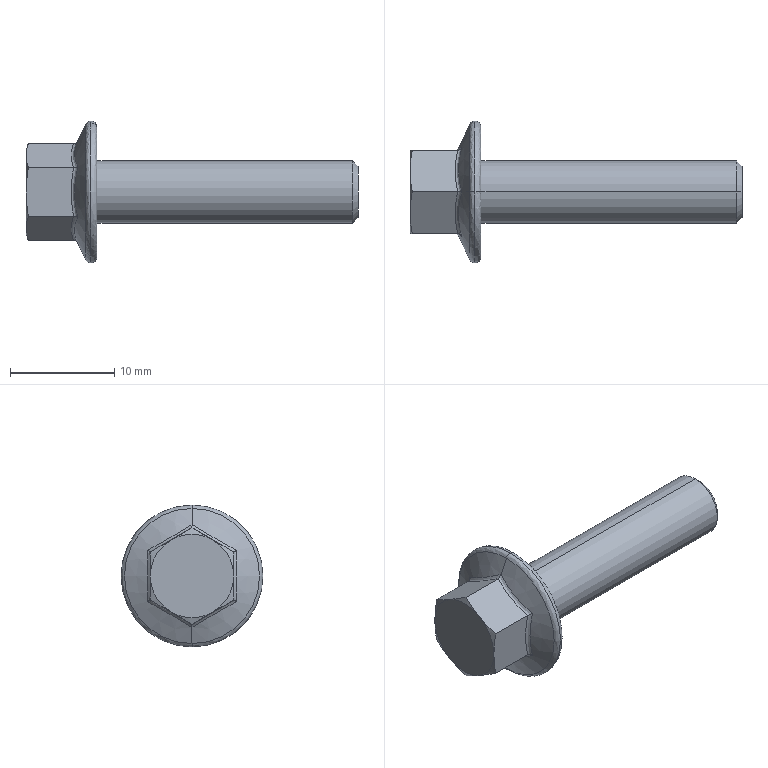Part | STEP file | hexagon flange bolts--small series gb_PreviewCfg | 1 solid | 31 faces | box 31.8 x 13.6 x 13.6 mm | volume 1212 mm3 | spline 10 | cone 10 | plane 9 | cylinder 2 | commonest cylinder face diameters 6 x2